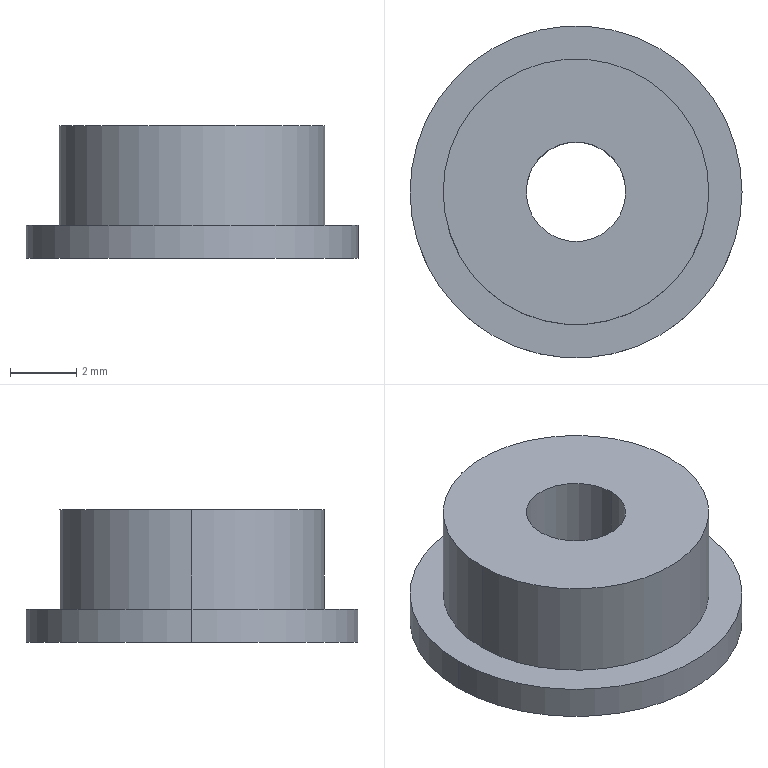Part | SolidWorks | features ICE 2, Extrusion 1 | 1 solid | 9 faces | box 10 x 10 x 4 mm | volume 201.062 mm3 | cylinder 6 | plane 3 | commonest cylinder face diameters 3 x2 8 x2 10 x2
STEP:
#1=CARTESIAN_POINT('',(-1.5,0.,0.));
#2=VERTEX_POINT('',#1);
#3=CARTESIAN_POINT('',(1.5,0.,0.));
#4=VERTEX_POINT('',#3);
#5=CARTESIAN_POINT('',(0.,0.,0.));
#6=DIRECTION('',(0.,0.,1.));
#7=DIRECTION('',(1.,0.,0.));
#8=AXIS2_PLACEMENT_3D('',#5,#6,#7);
#9=CIRCLE('',#8,1.5);
#10=EDGE_CURVE('',#2,#4,#9,.T.);
#11=ORIENTED_EDGE('',*,*,#10,.F.);
#12=CARTESIAN_POINT('',(-1.5,0.,4.));
#13=VERTEX_POINT('',#12);
#14=CARTESIAN_POINT('',(-1.5,0.,0.));
#15=DIRECTION('',(0.,0.,1.));
#16=VECTOR('',#15,1000.);
#17=LINE('',#14,#16);
#18=EDGE_CURVE('',#2,#13,#17,.T.);
#19=ORIENTED_EDGE('',*,*,#18,.T.);
#20=CARTESIAN_POINT('',(1.5,0.,4.));
#21=VERTEX_POINT('',#20);
#22=CARTESIAN_POINT('',(0.,0.,4.));
#23=DIRECTION('',(0.,0.,1.));
#24=DIRECTION('',(1.,0.,0.));
#25=AXIS2_PLACEMENT_3D('',#22,#23,#24);
#26=CIRCLE('',#25,1.5);
#27=EDGE_CURVE('',#13,#21,#26,.T.);
#28=ORIENTED_EDGE('',*,*,#27,.T.);
#29=CARTESIAN_POINT('',(1.5,0.,0.));
#30=DIRECTION('',(0.,0.,1.));
#31=VECTOR('',#30,1000.);
#32=LINE('',#29,#31);
#33=EDGE_CURVE('',#4,#21,#32,.T.);
#34=ORIENTED_EDGE('',*,*,#33,.F.);
#35=EDGE_LOOP('',(#11,#19,#28,#34));
#36=FACE_OUTER_BOUND('',#35,.T.);
#37=CARTESIAN_POINT('',(0.,0.,0.));
#38=DIRECTION('',(0.,0.,1.));
#39=DIRECTION('',(1.,0.,0.));
#40=AXIS2_PLACEMENT_3D('',#37,#38,#39);
#41=CYLINDRICAL_SURFACE('',#40,1.5);
#42=ADVANCED_FACE('',(#36),#41,.F.);
#43=CARTESIAN_POINT('',(4.,0.,1.));
#44=VERTEX_POINT('',#43);
#45=CARTESIAN_POINT('',(-4.,0.,1.));
#46=VERTEX_POINT('',#45);
#47=CARTESIAN_POINT('',(0.,0.,1.));
#48=DIRECTION('',(0.,0.,1.));
#49=DIRECTION('',(1.,0.,0.));
#50=AXIS2_PLACEMENT_3D('',#47,#48,#49);
#51=CIRCLE('',#50,4.);
#52=EDGE_CURVE('',#44,#46,#51,.T.);
#53=ORIENTED_EDGE('',*,*,#52,.T.);
#54=CARTESIAN_POINT('',(-4.,0.,4.));
#55=VERTEX_POINT('',#54);
#56=CARTESIAN_POINT('',(-4.,0.,1.));
#57=DIRECTION('',(0.,0.,1.));
#58=VECTOR('',#57,1000.);
#59=LINE('',#56,#58);
#60=EDGE_CURVE('',#46,#55,#59,.T.);
#61=ORIENTED_EDGE('',*,*,#60,.T.);
#62=CARTESIAN_POINT('',(4.,0.,4.));
#63=VERTEX_POINT('',#62);
#64=CARTESIAN_POINT('',(0.,0.,4.));
#65=DIRECTION('',(0.,0.,1.));
#66=DIRECTION('',(1.,0.,0.));
#67=AXIS2_PLACEMENT_3D('',#64,#65,#66);
#68=CIRCLE('',#67,4.);
#69=EDGE_CURVE('',#63,#55,#68,.T.);
#70=ORIENTED_EDGE('',*,*,#69,.F.);
#71=CARTESIAN_POINT('',(4.,0.,1.));
#72=DIRECTION('',(0.,0.,1.));
#73=VECTOR('',#72,1000.);
#74=LINE('',#71,#73);
#75=EDGE_CURVE('',#44,#63,#74,.T.);
#76=ORIENTED_EDGE('',*,*,#75,.F.);
#77=EDGE_LOOP('',(#53,#61,#70,#76));
#78=FACE_OUTER_BOUND('',#77,.T.);
#79=CARTESIAN_POINT('',(0.,0.,1.));
#80=DIRECTION('',(0.,0.,1.));
#81=DIRECTION('',(1.,0.,0.));
#82=AXIS2_PLACEMENT_3D('',#79,#80,#81);
#83=CYLINDRICAL_SURFACE('',#82,4.);
#84=ADVANCED_FACE('',(#78),#83,.T.);
#85=CARTESIAN_POINT('',(5.,0.,1.));
#86=VERTEX_POINT('',#85);
#87=CARTESIAN_POINT('',(-5.,0.,1.));
#88=VERTEX_POINT('',#87);
#89=CARTESIAN_POINT('',(0.,0.,1.));
#90=DIRECTION('',(0.,0.,1.));
#91=DIRECTION('',(1.,0.,0.));
#92=AXIS2_PLACEMENT_3D('',#89,#90,#91);
#93=CIRCLE('',#92,5.);
#94=EDGE_CURVE('',#86,#88,#93,.T.);
#95=ORIENTED_EDGE('',*,*,#94,.F.);
#96=CARTESIAN_POINT('',(5.,0.,0.));
#97=VERTEX_POINT('',#96);
#98=CARTESIAN_POINT('',(5.,0.,4.));
#99=DIRECTION('',(0.,0.,-1.));
#100=VECTOR('',#99,1000.);
#101=LINE('',#98,#100);
#102=EDGE_CURVE('',#86,#97,#101,.T.);
#103=ORIENTED_EDGE('',*,*,#102,.T.);
#104=CARTESIAN_POINT('',(-5.,0.,0.));
#105=VERTEX_POINT('',#104);
#106=CARTESIAN_POINT('',(0.,0.,0.));
#107=DIRECTION('',(0.,0.,1.));
#108=DIRECTION('',(1.,0.,0.));
#109=AXIS2_PLACEMENT_3D('',#106,#107,#108);
#110=CIRCLE('',#109,5.);
#111=EDGE_CURVE('',#97,#105,#110,.T.);
#112=ORIENTED_EDGE('',*,*,#111,.T.);
#113=CARTESIAN_POINT('',(-5.,0.,4.));
#114=DIRECTION('',(0.,0.,-1.));
#115=VECTOR('',#114,1000.);
#116=LINE('',#113,#115);
#117=EDGE_CURVE('',#88,#105,#116,.T.);
#118=ORIENTED_EDGE('',*,*,#117,.F.);
#119=EDGE_LOOP('',(#95,#103,#112,#118));
#120=FACE_OUTER_BOUND('',#119,.T.);
#121=CARTESIAN_POINT('',(0.,0.,4.));
#122=DIRECTION('',(0.,0.,-1.));
#123=DIRECTION('',(-1.,0.,0.));
#124=AXIS2_PLACEMENT_3D('',#121,#122,#123);
#125=CYLINDRICAL_SURFACE('',#124,5.);
#126=ADVANCED_FACE('',(#120),#125,.T.);
#127=ORIENTED_EDGE('',*,*,#102,.F.);
#128=CARTESIAN_POINT('',(0.,0.,1.));
#129=DIRECTION('',(0.,0.,1.));
#130=DIRECTION('',(1.,0.,0.));
#131=AXIS2_PLACEMENT_3D('',#128,#129,#130);
#132=CIRCLE('',#131,5.);
#133=EDGE_CURVE('',#88,#86,#132,.T.);
#134=ORIENTED_EDGE('',*,*,#133,.F.);
#135=ORIENTED_EDGE('',*,*,#117,.T.);
#136=CARTESIAN_POINT('',(0.,0.,0.));
#137=DIRECTION('',(0.,0.,1.));
#138=DIRECTION('',(1.,0.,0.));
#139=AXIS2_PLACEMENT_3D('',#136,#137,#138);
#140=CIRCLE('',#139,5.);
#141=EDGE_CURVE('',#105,#97,#140,.T.);
#142=ORIENTED_EDGE('',*,*,#141,.T.);
#143=EDGE_LOOP('',(#127,#134,#135,#142));
#144=FACE_OUTER_BOUND('',#143,.T.);
#145=CARTESIAN_POINT('',(0.,0.,4.));
#146=DIRECTION('',(0.,0.,-1.));
#147=DIRECTION('',(-1.,0.,0.));
#148=AXIS2_PLACEMENT_3D('',#145,#146,#147);
#149=CYLINDRICAL_SURFACE('',#148,5.);
#150=ADVANCED_FACE('',(#144),#149,.T.);
#151=CARTESIAN_POINT('',(0.,0.,0.));
#152=DIRECTION('',(0.,0.,1.));
#153=DIRECTION('',(1.,0.,0.));
#154=AXIS2_PLACEMENT_3D('',#151,#152,#153);
#155=CIRCLE('',#154,1.5);
#156=EDGE_CURVE('',#4,#2,#155,.T.);
#157=ORIENTED_EDGE('',*,*,#156,.T.);
#158=ORIENTED_EDGE('',*,*,#10,.T.);
#159=EDGE_LOOP('',(#157,#158));
#160=FACE_BOUND('',#159,.T.);
#161=ORIENTED_EDGE('',*,*,#141,.F.);
#162=ORIENTED_EDGE('',*,*,#111,.F.);
#163=EDGE_LOOP('',(#161,#162));
#164=FACE_OUTER_BOUND('',#163,.T.);
#165=CARTESIAN_POINT('',(0.,0.,0.));
#166=DIRECTION('',(0.,0.,1.));
#167=DIRECTION('',(1.,0.,0.));
#168=AXIS2_PLACEMENT_3D('',#165,#166,#167);
#169=PLANE('',#168);
#170=ADVANCED_FACE('',(#160,#164),#169,.F.);
#171=ORIENTED_EDGE('',*,*,#52,.F.);
#172=CARTESIAN_POINT('',(0.,0.,1.));
#173=DIRECTION('',(0.,0.,1.));
#174=DIRECTION('',(1.,0.,0.));
#175=AXIS2_PLACEMENT_3D('',#172,#173,#174);
#176=CIRCLE('',#175,4.);
#177=EDGE_CURVE('',#46,#44,#176,.T.);
#178=ORIENTED_EDGE('',*,*,#177,.F.);
#179=EDGE_LOOP('',(#171,#178));
#180=FACE_BOUND('',#179,.T.);
#181=ORIENTED_EDGE('',*,*,#133,.T.);
#182=ORIENTED_EDGE('',*,*,#94,.T.);
#183=EDGE_LOOP('',(#181,#182));
#184=FACE_OUTER_BOUND('',#183,.T.);
#185=CARTESIAN_POINT('',(0.,0.,1.));
#186=DIRECTION('',(0.,0.,1.));
#187=DIRECTION('',(1.,0.,0.));
#188=AXIS2_PLACEMENT_3D('',#185,#186,#187);
#189=PLANE('',#188);
#190=ADVANCED_FACE('',(#180,#184),#189,.T.);
#191=ORIENTED_EDGE('',*,*,#60,.F.);
#192=ORIENTED_EDGE('',*,*,#177,.T.);
#193=ORIENTED_EDGE('',*,*,#75,.T.);
#194=CARTESIAN_POINT('',(0.,0.,4.));
#195=DIRECTION('',(0.,0.,1.));
#196=DIRECTION('',(1.,0.,0.));
#197=AXIS2_PLACEMENT_3D('',#194,#195,#196);
#198=CIRCLE('',#197,4.);
#199=EDGE_CURVE('',#55,#63,#198,.T.);
#200=ORIENTED_EDGE('',*,*,#199,.F.);
#201=EDGE_LOOP('',(#191,#192,#193,#200));
#202=FACE_OUTER_BOUND('',#201,.T.);
#203=CARTESIAN_POINT('',(0.,0.,1.));
#204=DIRECTION('',(0.,0.,1.));
#205=DIRECTION('',(1.,0.,0.));
#206=AXIS2_PLACEMENT_3D('',#203,#204,#205);
#207=CYLINDRICAL_SURFACE('',#206,4.);
#208=ADVANCED_FACE('',(#202),#207,.T.);
#209=CARTESIAN_POINT('',(0.,0.,4.));
#210=DIRECTION('',(0.,0.,1.));
#211=DIRECTION('',(1.,0.,0.));
#212=AXIS2_PLACEMENT_3D('',#209,#210,#211);
#213=CIRCLE('',#212,1.5);
#214=EDGE_CURVE('',#21,#13,#213,.T.);
#215=ORIENTED_EDGE('',*,*,#214,.F.);
#216=ORIENTED_EDGE('',*,*,#27,.F.);
#217=EDGE_LOOP('',(#215,#216));
#218=FACE_BOUND('',#217,.T.);
#219=ORIENTED_EDGE('',*,*,#69,.T.);
#220=ORIENTED_EDGE('',*,*,#199,.T.);
#221=EDGE_LOOP('',(#219,#220));
#222=FACE_OUTER_BOUND('',#221,.T.);
#223=CARTESIAN_POINT('',(0.,0.,4.));
#224=DIRECTION('',(0.,0.,1.));
#225=DIRECTION('',(1.,0.,0.));
#226=AXIS2_PLACEMENT_3D('',#223,#224,#225);
#227=PLANE('',#226);
#228=ADVANCED_FACE('',(#218,#222),#227,.T.);
#229=ORIENTED_EDGE('',*,*,#18,.F.);
#230=ORIENTED_EDGE('',*,*,#156,.F.);
#231=ORIENTED_EDGE('',*,*,#33,.T.);
#232=ORIENTED_EDGE('',*,*,#214,.T.);
#233=EDGE_LOOP('',(#229,#230,#231,#232));
#234=FACE_OUTER_BOUND('',#233,.T.);
#235=CARTESIAN_POINT('',(0.,0.,0.));
#236=DIRECTION('',(0.,0.,1.));
#237=DIRECTION('',(1.,0.,0.));
#238=AXIS2_PLACEMENT_3D('',#235,#236,#237);
#239=CYLINDRICAL_SURFACE('',#238,1.5);
#240=ADVANCED_FACE('',(#234),#239,.F.);
#241=CLOSED_SHELL('',(#42,#84,#126,#150,#170,#190,#208,#228,#240));
#242=MANIFOLD_SOLID_BREP('',#241);
#243=CARTESIAN_POINT('',(0.,0.,0.));
#244=DIRECTION('',(0.,0.,1.));
#245=DIRECTION('',(1.,0.,0.));
#246=AXIS2_PLACEMENT_3D('',#243,#244,#245);
#247=(LENGTH_UNIT()NAMED_UNIT(*)SI_UNIT(.MILLI.,.METRE.));
#248=UNCERTAINTY_MEASURE_WITH_UNIT(LENGTH_MEASURE(0.00001),#247,'','');
#249=(NAMED_UNIT(*)PLANE_ANGLE_UNIT()SI_UNIT($,.RADIAN.));
#250=(NAMED_UNIT(*)SI_UNIT($,.STERADIAN.)SOLID_ANGLE_UNIT());
#251=(GEOMETRIC_REPRESENTATION_CONTEXT(3)GLOBAL_UNCERTAINTY_ASSIGNED_CONTEXT((#248))GLOBAL_UNIT_ASSIGNED_CONTEXT((#247,#249,#250))REPRESENTATION_CONTEXT('',''));
#252=ADVANCED_BREP_SHAPE_REPRESENTATION('',(#242,#246),#251);